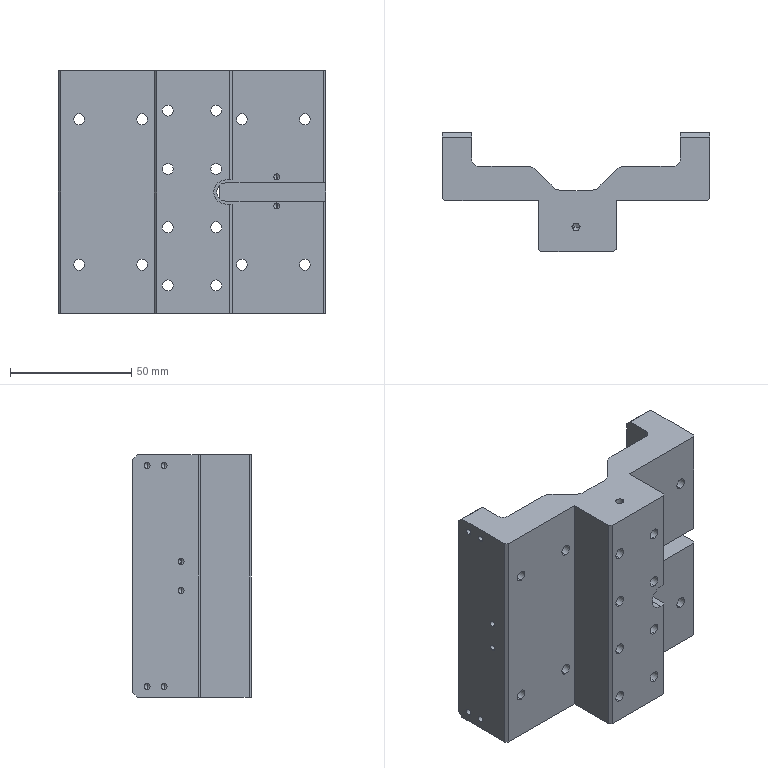Part | SolidWorks | features BaseBody 1 | 1 solid | 254 faces | box 110 x 49 x 100 mm | volume 206200 mm3 | cylinder 136 | plane 62 | cone 56 | commonest cylinder face diameters 4.5 x32 8 x32 2.5 x24 4.2 x16 6 x10 10 x9